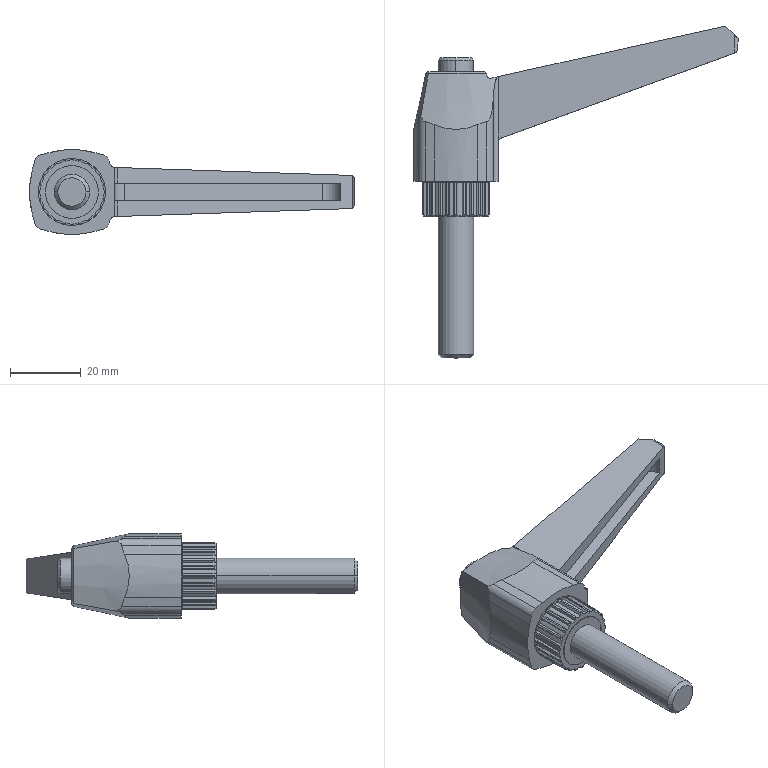Part | SolidWorks | features ICE 2, BaseBody 1, Chamfer 1 | 1 solid | 200 faces | box 92 x 94 x 24 mm | volume 28116 mm3 | plane 87 | cylinder 77 | cone 36 | commonest cylinder face diameters 19 x27 17.812 x14 17.813 x10 5.04 x4 10 x4 49.729 x4